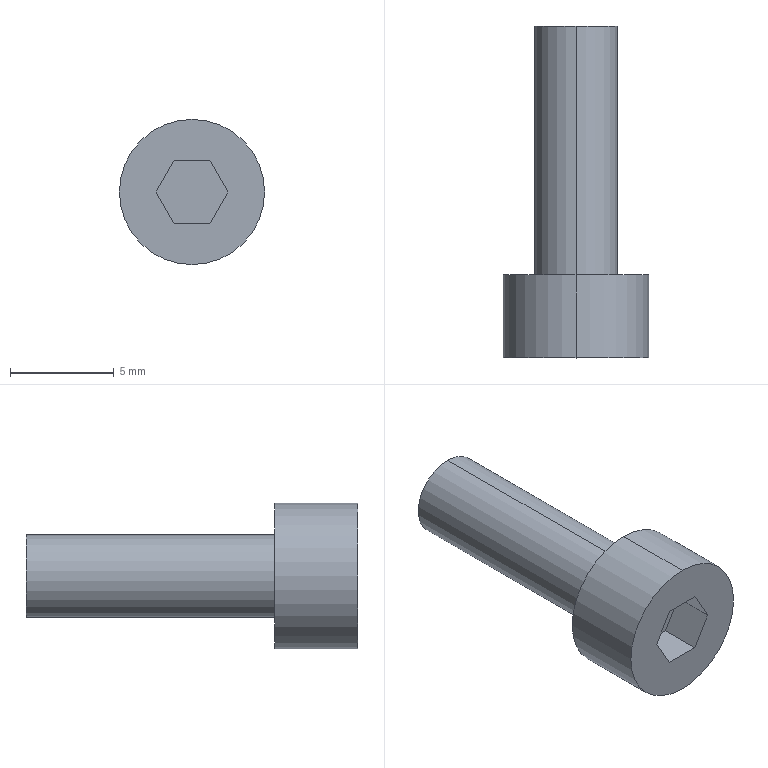Part | SolidWorks | features BaseBody 1 | 1 solid | 14 faces | box 7 x 16 x 7 mm | volume 289.146 mm3 | plane 10 | cylinder 4 | commonest cylinder face diameters 4 x2 7 x2
STEP:
#1=CARTESIAN_POINT('',(0.,16.,-2.));
#2=VERTEX_POINT('',#1);
#3=CARTESIAN_POINT('',(0.,16.,2.));
#4=VERTEX_POINT('',#3);
#5=CARTESIAN_POINT('',(0.,16.,0.));
#6=DIRECTION('',(0.,-1.,0.));
#7=DIRECTION('',(0.,0.,-1.));
#8=AXIS2_PLACEMENT_3D('',#5,#6,#7);
#9=CIRCLE('',#8,2.);
#10=EDGE_CURVE('',#2,#4,#9,.T.);
#11=ORIENTED_EDGE('',*,*,#10,.T.);
#12=CARTESIAN_POINT('',(0.,4.,2.));
#13=VERTEX_POINT('',#12);
#14=CARTESIAN_POINT('',(0.,16.,2.));
#15=DIRECTION('',(0.,-1.,0.));
#16=VECTOR('',#15,1000.);
#17=LINE('',#14,#16);
#18=EDGE_CURVE('',#4,#13,#17,.T.);
#19=ORIENTED_EDGE('',*,*,#18,.T.);
#20=CARTESIAN_POINT('',(0.,4.,-2.));
#21=VERTEX_POINT('',#20);
#22=CARTESIAN_POINT('',(0.,4.,0.));
#23=DIRECTION('',(0.,1.,0.));
#24=DIRECTION('',(0.,0.,-1.));
#25=AXIS2_PLACEMENT_3D('',#22,#23,#24);
#26=CIRCLE('',#25,2.);
#27=EDGE_CURVE('',#13,#21,#26,.T.);
#28=ORIENTED_EDGE('',*,*,#27,.T.);
#29=CARTESIAN_POINT('',(0.,16.,-2.));
#30=DIRECTION('',(0.,-1.,0.));
#31=VECTOR('',#30,1000.);
#32=LINE('',#29,#31);
#33=EDGE_CURVE('',#2,#21,#32,.T.);
#34=ORIENTED_EDGE('',*,*,#33,.F.);
#35=EDGE_LOOP('',(#11,#19,#28,#34));
#36=FACE_OUTER_BOUND('',#35,.T.);
#37=CARTESIAN_POINT('',(0.,16.,0.));
#38=DIRECTION('',(0.,-1.,0.));
#39=DIRECTION('',(0.,0.,-1.));
#40=AXIS2_PLACEMENT_3D('',#37,#38,#39);
#41=CYLINDRICAL_SURFACE('',#40,2.);
#42=ADVANCED_FACE('',(#36),#41,.T.);
#43=CARTESIAN_POINT('',(0.,4.,3.5));
#44=VERTEX_POINT('',#43);
#45=CARTESIAN_POINT('',(0.,4.,-3.5));
#46=VERTEX_POINT('',#45);
#47=CARTESIAN_POINT('',(0.,4.,0.));
#48=DIRECTION('',(0.,1.,0.));
#49=DIRECTION('',(0.,0.,-1.));
#50=AXIS2_PLACEMENT_3D('',#47,#48,#49);
#51=CIRCLE('',#50,3.5);
#52=EDGE_CURVE('',#44,#46,#51,.T.);
#53=ORIENTED_EDGE('',*,*,#52,.F.);
#54=CARTESIAN_POINT('',(0.,0.,3.5));
#55=VERTEX_POINT('',#54);
#56=CARTESIAN_POINT('',(0.,4.,3.5));
#57=DIRECTION('',(0.,-1.,0.));
#58=VECTOR('',#57,1000.);
#59=LINE('',#56,#58);
#60=EDGE_CURVE('',#44,#55,#59,.T.);
#61=ORIENTED_EDGE('',*,*,#60,.T.);
#62=CARTESIAN_POINT('',(0.,0.,-3.5));
#63=VERTEX_POINT('',#62);
#64=CARTESIAN_POINT('',(0.,0.,0.));
#65=DIRECTION('',(0.,1.,0.));
#66=DIRECTION('',(0.,0.,-1.));
#67=AXIS2_PLACEMENT_3D('',#64,#65,#66);
#68=CIRCLE('',#67,3.5);
#69=EDGE_CURVE('',#55,#63,#68,.T.);
#70=ORIENTED_EDGE('',*,*,#69,.T.);
#71=CARTESIAN_POINT('',(0.,4.,-3.5));
#72=DIRECTION('',(0.,-1.,0.));
#73=VECTOR('',#72,1000.);
#74=LINE('',#71,#73);
#75=EDGE_CURVE('',#46,#63,#74,.T.);
#76=ORIENTED_EDGE('',*,*,#75,.F.);
#77=EDGE_LOOP('',(#53,#61,#70,#76));
#78=FACE_OUTER_BOUND('',#77,.T.);
#79=CARTESIAN_POINT('',(0.,4.,0.));
#80=DIRECTION('',(0.,-1.,0.));
#81=DIRECTION('',(0.,0.,-1.));
#82=AXIS2_PLACEMENT_3D('',#79,#80,#81);
#83=CYLINDRICAL_SURFACE('',#82,3.5);
#84=ADVANCED_FACE('',(#78),#83,.T.);
#85=ORIENTED_EDGE('',*,*,#18,.F.);
#86=CARTESIAN_POINT('',(0.,16.,0.));
#87=DIRECTION('',(0.,-1.,0.));
#88=DIRECTION('',(0.,0.,-1.));
#89=AXIS2_PLACEMENT_3D('',#86,#87,#88);
#90=CIRCLE('',#89,2.);
#91=EDGE_CURVE('',#4,#2,#90,.T.);
#92=ORIENTED_EDGE('',*,*,#91,.T.);
#93=ORIENTED_EDGE('',*,*,#33,.T.);
#94=CARTESIAN_POINT('',(0.,4.,0.));
#95=DIRECTION('',(0.,1.,0.));
#96=DIRECTION('',(0.,0.,-1.));
#97=AXIS2_PLACEMENT_3D('',#94,#95,#96);
#98=CIRCLE('',#97,2.);
#99=EDGE_CURVE('',#21,#13,#98,.T.);
#100=ORIENTED_EDGE('',*,*,#99,.T.);
#101=EDGE_LOOP('',(#85,#92,#93,#100));
#102=FACE_OUTER_BOUND('',#101,.T.);
#103=CARTESIAN_POINT('',(0.,16.,0.));
#104=DIRECTION('',(0.,-1.,0.));
#105=DIRECTION('',(0.,0.,-1.));
#106=AXIS2_PLACEMENT_3D('',#103,#104,#105);
#107=CYLINDRICAL_SURFACE('',#106,2.);
#108=ADVANCED_FACE('',(#102),#107,.T.);
#109=CARTESIAN_POINT('',(0.,4.,0.));
#110=DIRECTION('',(0.,1.,0.));
#111=DIRECTION('',(0.,0.,-1.));
#112=AXIS2_PLACEMENT_3D('',#109,#110,#111);
#113=CIRCLE('',#112,3.5);
#114=EDGE_CURVE('',#46,#44,#113,.T.);
#115=ORIENTED_EDGE('',*,*,#114,.T.);
#116=ORIENTED_EDGE('',*,*,#52,.T.);
#117=EDGE_LOOP('',(#115,#116));
#118=FACE_OUTER_BOUND('',#117,.T.);
#119=ORIENTED_EDGE('',*,*,#99,.F.);
#120=ORIENTED_EDGE('',*,*,#27,.F.);
#121=EDGE_LOOP('',(#119,#120));
#122=FACE_BOUND('',#121,.T.);
#123=CARTESIAN_POINT('',(0.,4.,0.));
#124=DIRECTION('',(0.,1.,0.));
#125=DIRECTION('',(0.,0.,1.));
#126=AXIS2_PLACEMENT_3D('',#123,#124,#125);
#127=PLANE('',#126);
#128=ADVANCED_FACE('',(#118,#122),#127,.T.);
#129=ORIENTED_EDGE('',*,*,#10,.F.);
#130=ORIENTED_EDGE('',*,*,#91,.F.);
#131=EDGE_LOOP('',(#129,#130));
#132=FACE_OUTER_BOUND('',#131,.T.);
#133=CARTESIAN_POINT('',(0.,16.,0.));
#134=DIRECTION('',(0.,1.,0.));
#135=DIRECTION('',(0.,0.,1.));
#136=AXIS2_PLACEMENT_3D('',#133,#134,#135);
#137=PLANE('',#136);
#138=ADVANCED_FACE('',(#132),#137,.T.);
#139=ORIENTED_EDGE('',*,*,#60,.F.);
#140=ORIENTED_EDGE('',*,*,#114,.F.);
#141=ORIENTED_EDGE('',*,*,#75,.T.);
#142=CARTESIAN_POINT('',(0.,0.,0.));
#143=DIRECTION('',(0.,1.,0.));
#144=DIRECTION('',(0.,0.,-1.));
#145=AXIS2_PLACEMENT_3D('',#142,#143,#144);
#146=CIRCLE('',#145,3.5);
#147=EDGE_CURVE('',#63,#55,#146,.T.);
#148=ORIENTED_EDGE('',*,*,#147,.T.);
#149=EDGE_LOOP('',(#139,#140,#141,#148));
#150=FACE_OUTER_BOUND('',#149,.T.);
#151=CARTESIAN_POINT('',(0.,4.,0.));
#152=DIRECTION('',(0.,-1.,0.));
#153=DIRECTION('',(0.,0.,-1.));
#154=AXIS2_PLACEMENT_3D('',#151,#152,#153);
#155=CYLINDRICAL_SURFACE('',#154,3.5);
#156=ADVANCED_FACE('',(#150),#155,.T.);
#157=ORIENTED_EDGE('',*,*,#147,.F.);
#158=ORIENTED_EDGE('',*,*,#69,.F.);
#159=EDGE_LOOP('',(#157,#158));
#160=FACE_OUTER_BOUND('',#159,.T.);
#161=CARTESIAN_POINT('',(1.732,0.,0.));
#162=VERTEX_POINT('',#161);
#163=CARTESIAN_POINT('',(0.866,0.,-1.5));
#164=VERTEX_POINT('',#163);
#165=CARTESIAN_POINT('',(0.866,0.,-1.5));
#166=DIRECTION('',(-0.5,0.,-0.866));
#167=VECTOR('',#166,1000.);
#168=LINE('',#165,#167);
#169=EDGE_CURVE('',#162,#164,#168,.T.);
#170=ORIENTED_EDGE('',*,*,#169,.T.);
#171=CARTESIAN_POINT('',(-0.866,0.,-1.5));
#172=VERTEX_POINT('',#171);
#173=CARTESIAN_POINT('',(-0.866,0.,-1.5));
#174=DIRECTION('',(-1.,0.,0.));
#175=VECTOR('',#174,1000.);
#176=LINE('',#173,#175);
#177=EDGE_CURVE('',#164,#172,#176,.T.);
#178=ORIENTED_EDGE('',*,*,#177,.T.);
#179=CARTESIAN_POINT('',(-1.732,0.,0.));
#180=VERTEX_POINT('',#179);
#181=CARTESIAN_POINT('',(-1.732,0.,0.));
#182=DIRECTION('',(-0.5,0.,0.866));
#183=VECTOR('',#182,1000.);
#184=LINE('',#181,#183);
#185=EDGE_CURVE('',#172,#180,#184,.T.);
#186=ORIENTED_EDGE('',*,*,#185,.T.);
#187=CARTESIAN_POINT('',(-0.866,0.,1.5));
#188=VERTEX_POINT('',#187);
#189=CARTESIAN_POINT('',(-0.866,0.,1.5));
#190=DIRECTION('',(0.5,0.,0.866));
#191=VECTOR('',#190,1000.);
#192=LINE('',#189,#191);
#193=EDGE_CURVE('',#180,#188,#192,.T.);
#194=ORIENTED_EDGE('',*,*,#193,.T.);
#195=CARTESIAN_POINT('',(0.866,0.,1.5));
#196=VERTEX_POINT('',#195);
#197=CARTESIAN_POINT('',(0.866,0.,1.5));
#198=DIRECTION('',(1.,0.,0.));
#199=VECTOR('',#198,1000.);
#200=LINE('',#197,#199);
#201=EDGE_CURVE('',#188,#196,#200,.T.);
#202=ORIENTED_EDGE('',*,*,#201,.T.);
#203=CARTESIAN_POINT('',(1.732,0.,0.));
#204=DIRECTION('',(-0.5,0.,0.866));
#205=VECTOR('',#204,1000.);
#206=LINE('',#203,#205);
#207=EDGE_CURVE('',#162,#196,#206,.T.);
#208=ORIENTED_EDGE('',*,*,#207,.F.);
#209=EDGE_LOOP('',(#170,#178,#186,#194,#202,#208));
#210=FACE_BOUND('',#209,.T.);
#211=CARTESIAN_POINT('',(0.,0.,0.));
#212=DIRECTION('',(0.,1.,0.));
#213=DIRECTION('',(0.,0.,1.));
#214=AXIS2_PLACEMENT_3D('',#211,#212,#213);
#215=PLANE('',#214);
#216=ADVANCED_FACE('',(#160,#210),#215,.F.);
#217=CARTESIAN_POINT('',(0.866,2.,1.5));
#218=VERTEX_POINT('',#217);
#219=CARTESIAN_POINT('',(0.866,2.,1.5));
#220=DIRECTION('',(0.,-1.,0.));
#221=VECTOR('',#220,1000.);
#222=LINE('',#219,#221);
#223=EDGE_CURVE('',#218,#196,#222,.T.);
#224=ORIENTED_EDGE('',*,*,#223,.F.);
#225=CARTESIAN_POINT('',(1.732,2.,0.));
#226=VERTEX_POINT('',#225);
#227=CARTESIAN_POINT('',(1.732,2.,0.));
#228=DIRECTION('',(-0.5,0.,0.866));
#229=VECTOR('',#228,1000.);
#230=LINE('',#227,#229);
#231=EDGE_CURVE('',#226,#218,#230,.T.);
#232=ORIENTED_EDGE('',*,*,#231,.F.);
#233=CARTESIAN_POINT('',(1.732,2.,0.));
#234=DIRECTION('',(0.,1.,0.));
#235=VECTOR('',#234,1000.);
#236=LINE('',#233,#235);
#237=EDGE_CURVE('',#162,#226,#236,.T.);
#238=ORIENTED_EDGE('',*,*,#237,.F.);
#239=ORIENTED_EDGE('',*,*,#207,.T.);
#240=EDGE_LOOP('',(#224,#232,#238,#239));
#241=FACE_OUTER_BOUND('',#240,.T.);
#242=CARTESIAN_POINT('',(1.732,2.,0.));
#243=DIRECTION('',(0.866,0.,0.5));
#244=DIRECTION('',(0.5,0.,-0.866));
#245=AXIS2_PLACEMENT_3D('',#242,#243,#244);
#246=PLANE('',#245);
#247=ADVANCED_FACE('',(#241),#246,.F.);
#248=CARTESIAN_POINT('',(-0.866,2.,1.5));
#249=VERTEX_POINT('',#248);
#250=CARTESIAN_POINT('',(-0.866,2.,1.5));
#251=DIRECTION('',(0.,-1.,0.));
#252=VECTOR('',#251,1000.);
#253=LINE('',#250,#252);
#254=EDGE_CURVE('',#249,#188,#253,.T.);
#255=ORIENTED_EDGE('',*,*,#254,.F.);
#256=CARTESIAN_POINT('',(0.866,2.,1.5));
#257=DIRECTION('',(-1.,0.,0.));
#258=VECTOR('',#257,1000.);
#259=LINE('',#256,#258);
#260=EDGE_CURVE('',#218,#249,#259,.T.);
#261=ORIENTED_EDGE('',*,*,#260,.F.);
#262=ORIENTED_EDGE('',*,*,#223,.T.);
#263=ORIENTED_EDGE('',*,*,#201,.F.);
#264=EDGE_LOOP('',(#255,#261,#262,#263));
#265=FACE_OUTER_BOUND('',#264,.T.);
#266=CARTESIAN_POINT('',(0.866,2.,1.5));
#267=DIRECTION('',(0.,0.,1.));
#268=DIRECTION('',(1.,0.,0.));
#269=AXIS2_PLACEMENT_3D('',#266,#267,#268);
#270=PLANE('',#269);
#271=ADVANCED_FACE('',(#265),#270,.F.);
#272=CARTESIAN_POINT('',(-1.732,2.,0.));
#273=VERTEX_POINT('',#272);
#274=CARTESIAN_POINT('',(-0.866,2.,-1.5));
#275=VERTEX_POINT('',#274);
#276=CARTESIAN_POINT('',(-1.732,2.,0.));
#277=DIRECTION('',(0.5,0.,-0.866));
#278=VECTOR('',#277,1000.);
#279=LINE('',#276,#278);
#280=EDGE_CURVE('',#273,#275,#279,.T.);
#281=ORIENTED_EDGE('',*,*,#280,.T.);
#282=CARTESIAN_POINT('',(0.866,2.,-1.5));
#283=VERTEX_POINT('',#282);
#284=CARTESIAN_POINT('',(-0.866,2.,-1.5));
#285=DIRECTION('',(1.,0.,0.));
#286=VECTOR('',#285,1000.);
#287=LINE('',#284,#286);
#288=EDGE_CURVE('',#275,#283,#287,.T.);
#289=ORIENTED_EDGE('',*,*,#288,.T.);
#290=CARTESIAN_POINT('',(0.866,2.,-1.5));
#291=DIRECTION('',(0.5,0.,0.866));
#292=VECTOR('',#291,1000.);
#293=LINE('',#290,#292);
#294=EDGE_CURVE('',#283,#226,#293,.T.);
#295=ORIENTED_EDGE('',*,*,#294,.T.);
#296=ORIENTED_EDGE('',*,*,#231,.T.);
#297=ORIENTED_EDGE('',*,*,#260,.T.);
#298=CARTESIAN_POINT('',(-0.866,2.,1.5));
#299=DIRECTION('',(-0.5,0.,-0.866));
#300=VECTOR('',#299,1000.);
#301=LINE('',#298,#300);
#302=EDGE_CURVE('',#249,#273,#301,.T.);
#303=ORIENTED_EDGE('',*,*,#302,.T.);
#304=EDGE_LOOP('',(#281,#289,#295,#296,#297,#303));
#305=FACE_OUTER_BOUND('',#304,.T.);
#306=CARTESIAN_POINT('',(0.,2.,0.));
#307=DIRECTION('',(0.,-1.,0.));
#308=DIRECTION('',(0.,0.,-1.));
#309=AXIS2_PLACEMENT_3D('',#306,#307,#308);
#310=PLANE('',#309);
#311=ADVANCED_FACE('',(#305),#310,.T.);
#312=ORIENTED_EDGE('',*,*,#237,.T.);
#313=ORIENTED_EDGE('',*,*,#294,.F.);
#314=CARTESIAN_POINT('',(0.866,2.,-1.5));
#315=DIRECTION('',(0.,1.,0.));
#316=VECTOR('',#315,1000.);
#317=LINE('',#314,#316);
#318=EDGE_CURVE('',#164,#283,#317,.T.);
#319=ORIENTED_EDGE('',*,*,#318,.F.);
#320=ORIENTED_EDGE('',*,*,#169,.F.);
#321=EDGE_LOOP('',(#312,#313,#319,#320));
#322=FACE_OUTER_BOUND('',#321,.T.);
#323=CARTESIAN_POINT('',(0.866,2.,-1.5));
#324=DIRECTION('',(0.866,0.,-0.5));
#325=DIRECTION('',(-0.5,0.,-0.866));
#326=AXIS2_PLACEMENT_3D('',#323,#324,#325);
#327=PLANE('',#326);
#328=ADVANCED_FACE('',(#322),#327,.F.);
#329=CARTESIAN_POINT('',(-1.732,2.,0.));
#330=DIRECTION('',(0.,-1.,0.));
#331=VECTOR('',#330,1000.);
#332=LINE('',#329,#331);
#333=EDGE_CURVE('',#273,#180,#332,.T.);
#334=ORIENTED_EDGE('',*,*,#333,.F.);
#335=ORIENTED_EDGE('',*,*,#302,.F.);
#336=ORIENTED_EDGE('',*,*,#254,.T.);
#337=ORIENTED_EDGE('',*,*,#193,.F.);
#338=EDGE_LOOP('',(#334,#335,#336,#337));
#339=FACE_OUTER_BOUND('',#338,.T.);
#340=CARTESIAN_POINT('',(-0.866,2.,1.5));
#341=DIRECTION('',(-0.866,0.,0.5));
#342=DIRECTION('',(0.5,0.,0.866));
#343=AXIS2_PLACEMENT_3D('',#340,#341,#342);
#344=PLANE('',#343);
#345=ADVANCED_FACE('',(#339),#344,.F.);
#346=ORIENTED_EDGE('',*,*,#318,.T.);
#347=ORIENTED_EDGE('',*,*,#288,.F.);
#348=CARTESIAN_POINT('',(-0.866,2.,-1.5));
#349=DIRECTION('',(0.,1.,0.));
#350=VECTOR('',#349,1000.);
#351=LINE('',#348,#350);
#352=EDGE_CURVE('',#172,#275,#351,.T.);
#353=ORIENTED_EDGE('',*,*,#352,.F.);
#354=ORIENTED_EDGE('',*,*,#177,.F.);
#355=EDGE_LOOP('',(#346,#347,#353,#354));
#356=FACE_OUTER_BOUND('',#355,.T.);
#357=CARTESIAN_POINT('',(-0.866,2.,-1.5));
#358=DIRECTION('',(0.,0.,-1.));
#359=DIRECTION('',(-1.,0.,0.));
#360=AXIS2_PLACEMENT_3D('',#357,#358,#359);
#361=PLANE('',#360);
#362=ADVANCED_FACE('',(#356),#361,.F.);
#363=ORIENTED_EDGE('',*,*,#352,.T.);
#364=ORIENTED_EDGE('',*,*,#280,.F.);
#365=ORIENTED_EDGE('',*,*,#333,.T.);
#366=ORIENTED_EDGE('',*,*,#185,.F.);
#367=EDGE_LOOP('',(#363,#364,#365,#366));
#368=FACE_OUTER_BOUND('',#367,.T.);
#369=CARTESIAN_POINT('',(-1.732,2.,0.));
#370=DIRECTION('',(-0.866,0.,-0.5));
#371=DIRECTION('',(-0.5,0.,0.866));
#372=AXIS2_PLACEMENT_3D('',#369,#370,#371);
#373=PLANE('',#372);
#374=ADVANCED_FACE('',(#368),#373,.F.);
#375=CLOSED_SHELL('',(#42,#84,#108,#128,#138,#156,#216,#247,#271,#311,#328,#345,#362,#374));
#376=MANIFOLD_SOLID_BREP('',#375);
#377=CARTESIAN_POINT('',(0.,0.,0.));
#378=DIRECTION('',(0.,0.,1.));
#379=DIRECTION('',(1.,0.,0.));
#380=AXIS2_PLACEMENT_3D('',#377,#378,#379);
#381=(LENGTH_UNIT()NAMED_UNIT(*)SI_UNIT(.MILLI.,.METRE.));
#382=UNCERTAINTY_MEASURE_WITH_UNIT(LENGTH_MEASURE(0.00001),#381,'','');
#383=(NAMED_UNIT(*)PLANE_ANGLE_UNIT()SI_UNIT($,.RADIAN.));
#384=(NAMED_UNIT(*)SI_UNIT($,.STERADIAN.)SOLID_ANGLE_UNIT());
#385=(GEOMETRIC_REPRESENTATION_CONTEXT(3)GLOBAL_UNCERTAINTY_ASSIGNED_CONTEXT((#382))GLOBAL_UNIT_ASSIGNED_CONTEXT((#381,#383,#384))REPRESENTATION_CONTEXT('',''));
#386=ADVANCED_BREP_SHAPE_REPRESENTATION('',(#376,#380),#385);